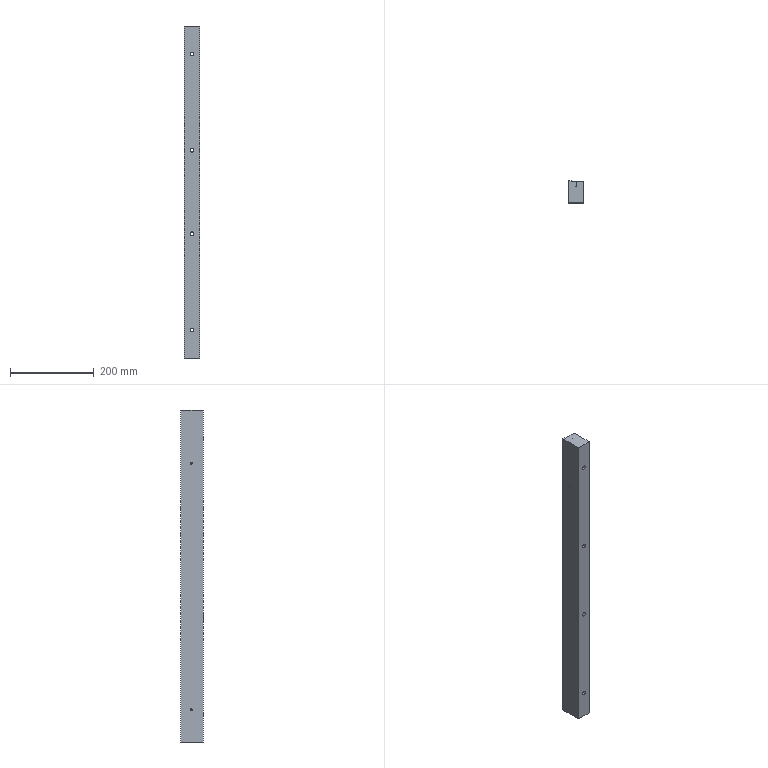Part | SolidWorks | features HoleWzd 4, Extrusion 1, LPattern 1 | 1 solid | 96 faces | box 36 x 53.5 x 794 mm | volume 1434418 mm3 | cylinder 50 | cone 34 | plane 12 | commonest cylinder face diameters 5 x30 9 x8 15 x8 4.2 x4